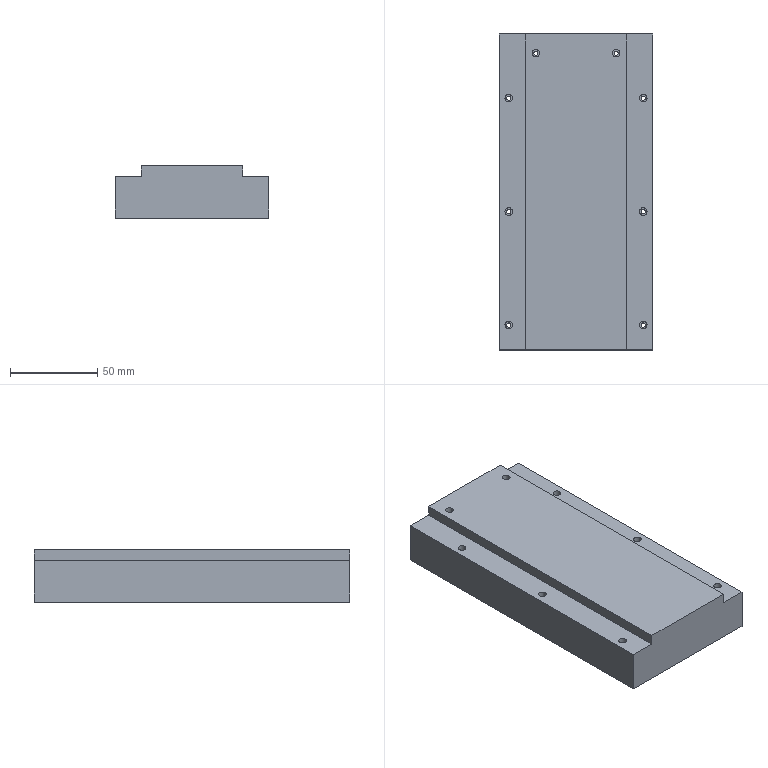NC program | NX | posted with a generic post | part box 88 x 181.05 x 30 mm
Lines 4247 to 5763 of 5763:
(PLANAR_MILL_3 , TOOL : D63_FACE_MILL)
N8480 T01 M6
N8482 G54
N8484 G17 G0 G90 X17.5 Y-153.525 S4500 M3
N8486 G43 Z20. H1
N8488 Z3.
N8490 G94 G1 Z0. F800.
N8492 Y-90.525
N8494 Y90.525
N8496 X-17.5
N8498 Y-90.525
N8500 Y-153.525
N8502 Z3.
N8504 G0 Z20.
N8506 M5
(PLANAR_MILL_4 , TOOL : D5-15-D6-50-3T-ROUGH)
N8508 T08 M6
N8510 G54
N8512 G17 G0 G90 X-25.04 Y69.397 S5000 M3
N8514 G43 Z20. H8
N8516 Z1.02
N8518 G94 G1 Z-0.98 F1500.
N8520 G3 X-27.04 Y71.397 R2.
N8522 G1 X-29.489
N8524 G3 X-30.889 Y69.997 R1.4
N8526 G1 Y67.548
N8528 G3 X-28.889 Y65.548 R2.
N8530 G1 Z1.02
N8532 G0 X-25.04 Y69.397 Z0.04
N8534 G1 Z-1.96
N8536 G3 X-27.04 Y71.397 R2.
N8538 G1 X-29.489
N8540 G3 X-30.889 Y69.997 R1.4
N8542 G1 Y67.548
N8544 G3 X-28.889 Y65.548 R2.
N8546 G1 Z0.04
N8548 G0 X-25.04 Y69.397 Z-0.94
N8550 G1 Z-2.94
N8552 G3 X-27.04 Y71.397 R2.
N8554 G1 X-29.489
N8556 G3 X-30.889 Y69.997 R1.4
N8558 G1 Y67.548
N8560 G3 X-28.889 Y65.548 R2.
N8562 G1 Z-0.94
N8564 G0 X-25.04 Y69.397 Z-1.92
N8566 G1 Z-3.92
N8568 G3 X-27.04 Y71.397 R2.
N8570 G1 X-29.489
N8572 G3 X-30.889 Y69.997 R1.4
N8574 G1 Y67.548
N8576 G3 X-28.889 Y65.548 R2.
N8578 G1 Z-1.92
N8580 G0 X-25.04 Y69.397 Z-2.9
N8582 G1 Z-4.9
N8584 G3 X-27.04 Y71.397 R2.
N8586 G1 X-29.489
N8588 G3 X-30.889 Y69.997 R1.4
N8590 G1 Y67.548
N8592 G3 X-28.889 Y65.548 R2.
N8594 G1 Z-2.9
N8596 G0 Z3.
N8598 Y28.051
N8600 Z1.02
N8602 G1 Z-0.98
N8604 G3 X-30.889 Y26.051 R2.
N8606 G1 Y23.602
N8608 G3 X-29.489 Y22.202 R1.4
N8610 G1 X-27.04
N8612 G3 X-25.04 Y24.202 R2.
N8614 G1 Z1.02
N8616 G0 X-28.889 Y28.051 Z0.04
N8618 G1 Z-1.96
N8620 G3 X-30.889 Y26.051 R2.
N8622 G1 Y23.602
N8624 G3 X-29.489 Y22.202 R1.4
N8626 G1 X-27.04
N8628 G3 X-25.04 Y24.202 R2.
N8630 G1 Z0.04
N8632 G0 X-28.889 Y28.051 Z-0.94
N8634 G1 Z-2.94
N8636 G3 X-30.889 Y26.051 R2.
N8638 G1 Y23.602
N8640 G3 X-29.489 Y22.202 R1.4
N8642 G1 X-27.04
N8644 G3 X-25.04 Y24.202 R2.
N8646 G1 Z-0.94
N8648 G0 X-28.889 Y28.051 Z-1.92
N8650 G1 Z-3.92
N8652 G3 X-30.889 Y26.051 R2.
N8654 G1 Y23.602
N8656 G3 X-29.489 Y22.202 R1.4
N8658 G1 X-27.04
N8660 G3 X-25.04 Y24.202 R2.
N8662 G1 Z-1.92
N8664 G0 X-28.889 Y28.051 Z-2.9
N8666 G1 Z-4.9
N8668 G3 X-30.889 Y26.051 R2.
N8670 G1 Y23.602
N8672 G3 X-29.489 Y22.202 R1.4
N8674 G1 X-27.04
N8676 G3 X-25.04 Y24.202 R2.
N8678 G1 Z-2.9
N8680 G0 Z3.
N8682 X24.773
N8684 Z1.02
N8686 G1 Z-0.98
N8688 G3 X26.773 Y22.202 R2.
N8690 G1 X29.222
N8692 G3 X30.622 Y23.602 R1.4
N8694 G1 Y26.051
N8696 G3 X28.622 Y28.051 R2.
N8698 G1 Z1.02
N8700 G0 X24.773 Y24.202 Z0.04
N8702 G1 Z-1.96
N8704 G3 X26.773 Y22.202 R2.
N8706 G1 X29.222
N8708 G3 X30.622 Y23.602 R1.4
N8710 G1 Y26.051
N8712 G3 X28.622 Y28.051 R2.
N8714 G1 Z0.04
N8716 G0 X24.773 Y24.202 Z-0.94
N8718 G1 Z-2.94
N8720 G3 X26.773 Y22.202 R2.
N8722 G1 X29.222
N8724 G3 X30.622 Y23.602 R1.4
N8726 G1 Y26.051
N8728 G3 X28.622 Y28.051 R2.
N8730 G1 Z-0.94
N8732 G0 X24.773 Y24.202 Z-1.92
N8734 G1 Z-3.92
N8736 G3 X26.773 Y22.202 R2.
N8738 G1 X29.222
N8740 G3 X30.622 Y23.602 R1.4
N8742 G1 Y26.051
N8744 G3 X28.622 Y28.051 R2.
N8746 G1 Z-1.92
N8748 G0 X24.773 Y24.202 Z-2.9
N8750 G1 Z-4.9
N8752 G3 X26.773 Y22.202 R2.
N8754 G1 X29.222
N8756 G3 X30.622 Y23.602 R1.4
N8758 G1 Y26.051
N8760 G3 X28.622 Y28.051 R2.
N8762 G1 Z-2.9
N8764 G0 Z3.
N8766 Y65.548
N8768 Z1.02
N8770 G1 Z-0.98
N8772 G3 X30.622 Y67.548 R2.
N8774 G1 Y69.997
N8776 G3 X29.222 Y71.397 R1.4
N8778 G1 X26.773
N8780 G3 X24.773 Y69.397 R2.
N8782 G1 Z1.02
N8784 G0 X28.622 Y65.548 Z0.04
N8786 G1 Z-1.96
N8788 G3 X30.622 Y67.548 R2.
N8790 G1 Y69.997
N8792 G3 X29.222 Y71.397 R1.4
N8794 G1 X26.773
N8796 G3 X24.773 Y69.397 R2.
N8798 G1 Z0.04
N8800 G0 X28.622 Y65.548 Z-0.94
N8802 G1 Z-2.94
N8804 G3 X30.622 Y67.548 R2.
N8806 G1 Y69.997
N8808 G3 X29.222 Y71.397 R1.4
N8810 G1 X26.773
N8812 G3 X24.773 Y69.397 R2.
N8814 G1 Z-0.94
N8816 G0 X28.622 Y65.548 Z-1.92
N8818 G1 Z-3.92
N8820 G3 X30.622 Y67.548 R2.
N8822 G1 Y69.997
N8824 G3 X29.222 Y71.397 R1.4
N8826 G1 X26.773
N8828 G3 X24.773 Y69.397 R2.
N8830 G1 Z-1.92
N8832 G0 X28.622 Y65.548 Z-2.9
N8834 G1 Z-4.9
N8836 G3 X30.622 Y67.548 R2.
N8838 G1 Y69.997
N8840 G3 X29.222 Y71.397 R1.4
N8842 G1 X26.773
N8844 G3 X24.773 Y69.397 R2.
N8846 G1 Z-2.9
N8848 G0 Z20.
(PLANAR_MILL_4_COPY , TOOL : D5-15-D6-50-3T-ROUGH)
N8850 X-13.196 Y12.175
N8852 Z1.5
N8854 G1 Z-0.5
N8856 G3 X-15.196 Y14.175 R2.
N8858 G1 X-18.072
N8860 G3 X-18.464 Y13.856 R0.4
N8862 G1 X-19.043 Y11.038
N8864 G3 X-17.487 Y8.676 R2.
N8866 G1 Z1.5
N8868 G0 Z20.
N8870 X17.487
N8872 Z1.5
N8874 G1 Z-0.5
N8876 G3 X19.043 Y11.038 R2.
N8878 G1 X18.464 Y13.856
N8880 G3 X18.072 Y14.175 R0.4
N8882 G1 X15.196
N8884 G3 X13.196 Y12.175 R2.
N8886 G1 Z1.5
N8888 G0 Z20.
N8890 X27.551 Y-68.925
N8892 Z1.5
N8894 G1 Z-0.5
N8896 G3 X29.551 Y-70.925 R2.
N8898 G1 X33.
N8900 G3 X33.4 Y-70.525 R0.4
N8902 G1 Y-67.076
N8904 G3 X31.4 Y-65.076 R2.
N8906 G1 Z1.5
N8908 G0 Z20.
N8910 X-31.4
N8912 Z1.5
N8914 G1 Z-0.5
N8916 G3 X-33.4 Y-67.076 R2.
N8918 G1 Y-70.525
N8920 G3 X-33. Y-70.925 R0.4
N8922 G1 X-29.551
N8924 G3 X-27.551 Y-68.925 R2.
N8926 G1 Z1.5
N8928 G0 Z20.
N8930 X-31.4 Y-65.076
N8932 Z1.
N8934 G1 Z-1.
N8936 G3 X-33.4 Y-67.076 R2.
N8938 G1 Y-70.525
N8940 G3 X-33. Y-70.925 R0.4
N8942 G1 X-29.551
N8944 G3 X-27.551 Y-68.925 R2.
N8946 G1 Z1.
N8948 G0 Z20.
N8950 X27.551
N8952 Z1.
N8954 G1 Z-1.
N8956 G3 X29.551 Y-70.925 R2.
N8958 G1 X33.
N8960 G3 X33.4 Y-70.525 R0.4
N8962 G1 Y-67.076
N8964 G3 X31.4 Y-65.076 R2.
N8966 G1 Z1.
N8968 G0 Z20.
N8970 X17.487 Y8.676
N8972 Z1.
N8974 G1 Z-1.
N8976 G3 X19.043 Y11.038 R2.
N8978 G1 X18.464 Y13.856
N8980 G3 X18.072 Y14.175 R0.4
N8982 G1 X15.196
N8984 G3 X13.196 Y12.175 R2.
N8986 G1 Z1.
N8988 G0 Z20.
N8990 X-13.196
N8992 Z1.
N8994 G1 Z-1.
N8996 G3 X-15.196 Y14.175 R2.
N8998 G1 X-18.072
N9000 G3 X-18.464 Y13.856 R0.4
N9002 G1 X-19.043 Y11.038
N9004 G3 X-17.487 Y8.676 R2.
N9006 G1 Z1.
N9008 G0 Z20.
N9010 X-13.196 Y12.175
N9012 Z0.5
N9014 G1 Z-1.5
N9016 G3 X-15.196 Y14.175 R2.
N9018 G1 X-18.072
N9020 G3 X-18.464 Y13.856 R0.4
N9022 G1 X-19.043 Y11.038
N9024 G3 X-17.487 Y8.676 R2.
N9026 G1 Z0.5
N9028 G0 Z20.
N9030 X17.487
N9032 Z0.5
N9034 G1 Z-1.5
N9036 G3 X19.043 Y11.038 R2.
N9038 G1 X18.464 Y13.856
N9040 G3 X18.072 Y14.175 R0.4
N9042 G1 X15.196
N9044 G3 X13.196 Y12.175 R2.
N9046 G1 Z0.5
N9048 G0 Z20.
N9050 X27.551 Y-68.925
N9052 Z0.5
N9054 G1 Z-1.5
N9056 G3 X29.551 Y-70.925 R2.
N9058 G1 X33.
N9060 G3 X33.4 Y-70.525 R0.4
N9062 G1 Y-67.076
N9064 G3 X31.4 Y-65.076 R2.
N9066 G1 Z0.5
N9068 G0 Z20.
N9070 X-31.4
N9072 Z0.5
N9074 G1 Z-1.5
N9076 G3 X-33.4 Y-67.076 R2.
N9078 G1 Y-70.525
N9080 G3 X-33. Y-70.925 R0.4
N9082 G1 X-29.551
N9084 G3 X-27.551 Y-68.925 R2.
N9086 G1 Z0.5
N9088 G0 Z20.
N9090 X-31.4 Y-65.076
N9092 Z0.4
N9094 G1 Z-1.6
N9096 G3 X-33.4 Y-67.076 R2.
N9098 G1 Y-70.525
N9100 G3 X-33. Y-70.925 R0.4
N9102 G1 X-29.551
N9104 G3 X-27.551 Y-68.925 R2.
N9106 G1 Z0.4
N9108 G0 Z20.
N9110 X27.551
N9112 Z0.4
N9114 G1 Z-1.6
N9116 G3 X29.551 Y-70.925 R2.
N9118 G1 X33.
N9120 G3 X33.4 Y-70.525 R0.4
N9122 G1 Y-67.076
N9124 G3 X31.4 Y-65.076 R2.
N9126 G1 Z0.4
N9128 G0 Z20.
N9130 X17.487 Y8.676
N9132 Z0.4
N9134 G1 Z-1.6
N9136 G3 X19.043 Y11.038 R2.
N9138 G1 X18.464 Y13.856
N9140 G3 X18.072 Y14.175 R0.4
N9142 G1 X15.196
N9144 G3 X13.196 Y12.175 R2.
N9146 G1 Z0.4
N9148 G0 Z20.
N9150 X-13.196
N9152 Z0.4
N9154 G1 Z-1.6
N9156 G3 X-15.196 Y14.175 R2.
N9158 G1 X-18.072
N9160 G3 X-18.464 Y13.856 R0.4
N9162 G1 X-19.043 Y11.038
N9164 G3 X-17.487 Y8.676 R2.
N9166 G1 Z0.4
N9168 G0 Z20.
(PLANAR_MILL_4_COPY_COPY , TOOL : D5-15-D6-50-3T-ROUGH)
N9170 X12.692 Y4.691
N9172 Z-0.696
N9174 G1 Z-2.696
N9176 G3 X14.248 Y7.053 R2.
N9178 G1 X13.668 Y9.871
N9180 G3 X13.277 Y10.19 R0.4
N9182 G1 X10.4
N9184 G3 X8.4 Y8.19 R2.
N9186 G1 Z-0.696
N9188 G0 X12.692 Y4.691 Z-1.691
N9190 G1 Z-3.691
N9192 G3 X14.248 Y7.053 R2.
N9194 G1 X13.668 Y9.871
N9196 G3 X13.277 Y10.19 R0.4
N9198 G1 X10.4
N9200 G3 X8.4 Y8.19 R2.
N9202 G1 Z-1.691
N9204 G0 X12.692 Y4.691 Z-2.687
N9206 G1 Z-4.687
N9208 G3 X14.248 Y7.053 R2.
N9210 G1 X13.668 Y9.871
N9212 G3 X13.277 Y10.19 R0.4
N9214 G1 X10.4
N9216 G3 X8.4 Y8.19 R2.
N9218 G1 Z-2.687
N9220 G0 X12.692 Y4.691 Z-3.683
N9222 G1 Z-5.683
N9224 G3 X14.248 Y7.053 R2.
N9226 G1 X13.668 Y9.871
N9228 G3 X13.277 Y10.19 R0.4
N9230 G1 X10.4
N9232 G3 X8.4 Y8.19 R2.
N9234 G1 Z-3.683
N9236 G0 X12.692 Y4.691 Z-4.678
N9238 G1 Z-6.678
N9240 G3 X14.248 Y7.053 R2.
N9242 G1 X13.668 Y9.871
N9244 G3 X13.277 Y10.19 R0.4
N9246 G1 X10.4
N9248 G3 X8.4 Y8.19 R2.
N9250 G1 Z-4.678
N9252 G0 X12.692 Y4.691 Z-5.674
N9254 G1 Z-7.674
N9256 G3 X14.248 Y7.053 R2.
N9258 G1 X13.668 Y9.871
N9260 G3 X13.277 Y10.19 R0.4
N9262 G1 X10.4
N9264 G3 X8.4 Y8.19 R2.
N9266 G1 Z-5.674
N9268 G0 X12.692 Y4.691 Z-6.67
N9270 G1 Z-8.67
N9272 G3 X14.248 Y7.053 R2.
N9274 G1 X13.668 Y9.871
N9276 G3 X13.277 Y10.19 R0.4
N9278 G1 X10.4
N9280 G3 X8.4 Y8.19 R2.
N9282 G1 Z-6.67
N9284 G0 X12.692 Y4.691 Z-7.665
N9286 G1 Z-9.665
N9288 G3 X14.248 Y7.053 R2.
N9290 G1 X13.668 Y9.871
N9292 G3 X13.277 Y10.19 R0.4
N9294 G1 X10.4
N9296 G3 X8.4 Y8.19 R2.
N9298 G1 Z-7.665
N9300 G0 X12.692 Y4.691 Z-8.661
N9302 G1 Z-10.661
N9304 G3 X14.248 Y7.053 R2.
N9306 G1 X13.668 Y9.871
N9308 G3 X13.277 Y10.19 R0.4
N9310 G1 X10.4
N9312 G3 X8.4 Y8.19 R2.
N9314 G1 Z-8.661
N9316 G0 X12.692 Y4.691 Z-9.657
N9318 G1 Z-11.657
N9320 G3 X14.248 Y7.053 R2.
N9322 G1 X13.668 Y9.871
N9324 G3 X13.277 Y10.19 R0.4
N9326 G1 X10.4
N9328 G3 X8.4 Y8.19 R2.
N9330 G1 Z-9.657
N9332 G0 X12.692 Y4.691 Z-10.652
N9334 G1 Z-12.652
N9336 G3 X14.248 Y7.053 R2.
N9338 G1 X13.668 Y9.871
N9340 G3 X13.277 Y10.19 R0.4
N9342 G1 X10.4
N9344 G3 X8.4 Y8.19 R2.
N9346 G1 Z-10.652
N9348 G0 X12.692 Y4.691 Z-11.648
N9350 G1 Z-13.648
N9352 G3 X14.248 Y7.053 R2.
N9354 G1 X13.668 Y9.871
N9356 G3 X13.277 Y10.19 R0.4
N9358 G1 X10.4
N9360 G3 X8.4 Y8.19 R2.
N9362 G1 Z-11.648
N9364 G0 X12.692 Y4.691 Z-12.643
N9366 G1 Z-14.643
N9368 G3 X14.248 Y7.053 R2.
N9370 G1 X13.668 Y9.871
N9372 G3 X13.277 Y10.19 R0.4
N9374 G1 X10.4
N9376 G3 X8.4 Y8.19 R2.
N9378 G1 Z-12.643
N9380 G0 X12.692 Y4.691 Z-13.639
N9382 G1 Z-15.639
N9384 G3 X14.248 Y7.053 R2.
N9386 G1 X13.668 Y9.871
N9388 G3 X13.277 Y10.19 R0.4
N9390 G1 X10.4
N9392 G3 X8.4 Y8.19 R2.
N9394 G1 Z-13.639
N9396 G0 X12.692 Y4.691 Z-14.635
N9398 G1 Z-16.635
N9400 G3 X14.248 Y7.053 R2.
N9402 G1 X13.668 Y9.871
N9404 G3 X13.277 Y10.19 R0.4
N9406 G1 X10.4
N9408 G3 X8.4 Y8.19 R2.
N9410 G1 Z-14.635
N9412 G0 X12.692 Y4.691 Z-15.63
N9414 G1 Z-17.63
N9416 G3 X14.248 Y7.053 R2.
N9418 G1 X13.668 Y9.871
N9420 G3 X13.277 Y10.19 R0.4
N9422 G1 X10.4
N9424 G3 X8.4 Y8.19 R2.
N9426 G1 Z-15.63
N9428 G0 X12.692 Y4.691 Z-16.626
N9430 G1 Z-18.626
N9432 G3 X14.248 Y7.053 R2.
N9434 G1 X13.668 Y9.871
N9436 G3 X13.277 Y10.19 R0.4
N9438 G1 X10.4
N9440 G3 X8.4 Y8.19 R2.
N9442 G1 Z-16.626
N9444 G0 X12.692 Y4.691 Z-17.622
N9446 G1 Z-19.622
N9448 G3 X14.248 Y7.053 R2.
N9450 G1 X13.668 Y9.871
N9452 G3 X13.277 Y10.19 R0.4
N9454 G1 X10.4
N9456 G3 X8.4 Y8.19 R2.
N9458 G1 Z-17.622
N9460 G0 X12.692 Y4.691 Z-18.617
N9462 G1 Z-20.617
N9464 G3 X14.248 Y7.053 R2.
N9466 G1 X13.668 Y9.871
N9468 G3 X13.277 Y10.19 R0.4
N9470 G1 X10.4
N9472 G3 X8.4 Y8.19 R2.
N9474 G1 Z-18.617
N9476 G0 X12.692 Y4.691 Z-19.613
N9478 G1 Z-21.613
N9480 G3 X14.248 Y7.053 R2.
N9482 G1 X13.668 Y9.871
N9484 G3 X13.277 Y10.19 R0.4
N9486 G1 X10.4
N9488 G3 X8.4 Y8.19 R2.
N9490 G1 Z-19.613
N9492 G0 X12.692 Y4.691 Z-20.609
N9494 G1 Z-22.609
N9496 G3 X14.248 Y7.053 R2.
N9498 G1 X13.668 Y9.871
N9500 G3 X13.277 Y10.19 R0.4
N9502 G1 X10.4
N9504 G3 X8.4 Y8.19 R2.
N9506 G1 Z-20.609
N9508 G0 X12.692 Y4.691 Z-21.604
N9510 G1 Z-23.604
N9512 G3 X14.248 Y7.053 R2.
N9514 G1 X13.668 Y9.871
N9516 G3 X13.277 Y10.19 R0.4
N9518 G1 X10.4
N9520 G3 X8.4 Y8.19 R2.
N9522 G1 Z-21.604
N9524 G0 X12.692 Y4.691 Z-22.6
N9526 G1 Z-24.6
N9528 G3 X14.248 Y7.053 R2.
N9530 G1 X13.668 Y9.871
N9532 G3 X13.277 Y10.19 R0.4
N9534 G1 X10.4
N9536 G3 X8.4 Y8.19 R2.
N9538 G1 Z-22.6
N9540 G0 Z1.3
N9542 X-8.4
N9544 Z-0.696
N9546 G1 Z-2.696
N9548 G3 X-10.4 Y10.19 R2.
N9550 G1 X-13.277
N9552 G3 X-13.668 Y9.871 R0.4
N9554 G1 X-14.248 Y7.053
N9556 G3 X-12.692 Y4.691 R2.
N9558 G1 Z-0.696
N9560 G0 X-8.4 Y8.19 Z-1.691
N9562 G1 Z-3.691
N9564 G3 X-10.4 Y10.19 R2.
N9566 G1 X-13.277
N9568 G3 X-13.668 Y9.871 R0.4
N9570 G1 X-14.248 Y7.053
N9572 G3 X-12.692 Y4.691 R2.
N9574 G1 Z-1.691
N9576 G0 X-8.4 Y8.19 Z-2.687
N9578 G1 Z-4.687
N9580 G3 X-10.4 Y10.19 R2.
N9582 G1 X-13.277
N9584 G3 X-13.668 Y9.871 R0.4
N9586 G1 X-14.248 Y7.053
N9588 G3 X-12.692 Y4.691 R2.
N9590 G1 Z-2.687
N9592 G0 X-8.4 Y8.19 Z-3.683
N9594 G1 Z-5.683
N9596 G3 X-10.4 Y10.19 R2.
N9598 G1 X-13.277
N9600 G3 X-13.668 Y9.871 R0.4
N9602 G1 X-14.248 Y7.053
N9604 G3 X-12.692 Y4.691 R2.
N9606 G1 Z-3.683
N9608 G0 X-8.4 Y8.19 Z-4.678
N9610 G1 Z-6.678
N9612 G3 X-10.4 Y10.19 R2.
N9614 G1 X-13.277
N9616 G3 X-13.668 Y9.871 R0.4
N9618 G1 X-14.248 Y7.053
N9620 G3 X-12.692 Y4.691 R2.
N9622 G1 Z-4.678
N9624 G0 X-8.4 Y8.19 Z-5.674
N9626 G1 Z-7.674
N9628 G3 X-10.4 Y10.19 R2.
N9630 G1 X-13.277
N9632 G3 X-13.668 Y9.871 R0.4
N9634 G1 X-14.248 Y7.053
N9636 G3 X-12.692 Y4.691 R2.
N9638 G1 Z-5.674
N9640 G0 X-8.4 Y8.19 Z-6.67
N9642 G1 Z-8.67
N9644 G3 X-10.4 Y10.19 R2.
N9646 G1 X-13.277
N9648 G3 X-13.668 Y9.871 R0.4
N9650 G1 X-14.248 Y7.053
N9652 G3 X-12.692 Y4.691 R2.
N9654 G1 Z-6.67
N9656 G0 X-8.4 Y8.19 Z-7.665
N9658 G1 Z-9.665
N9660 G3 X-10.4 Y10.19 R2.
N9662 G1 X-13.277
N9664 G3 X-13.668 Y9.871 R0.4
N9666 G1 X-14.248 Y7.053
N9668 G3 X-12.692 Y4.691 R2.
N9670 G1 Z-7.665
N9672 G0 X-8.4 Y8.19 Z-8.661
N9674 G1 Z-10.661
N9676 G3 X-10.4 Y10.19 R2.
N9678 G1 X-13.277
N9680 G3 X-13.668 Y9.871 R0.4
N9682 G1 X-14.248 Y7.053
N9684 G3 X-12.692 Y4.691 R2.
N9686 G1 Z-8.661
N9688 G0 X-8.4 Y8.19 Z-9.657
N9690 G1 Z-11.657
N9692 G3 X-10.4 Y10.19 R2.
N9694 G1 X-13.277
N9696 G3 X-13.668 Y9.871 R0.4
N9698 G1 X-14.248 Y7.053
N9700 G3 X-12.692 Y4.691 R2.
N9702 G1 Z-9.657
N9704 G0 X-8.4 Y8.19 Z-10.652
N9706 G1 Z-12.652
N9708 G3 X-10.4 Y10.19 R2.
N9710 G1 X-13.277
N9712 G3 X-13.668 Y9.871 R0.4
N9714 G1 X-14.248 Y7.053
N9716 G3 X-12.692 Y4.691 R2.
N9718 G1 Z-10.652
N9720 G0 X-8.4 Y8.19 Z-11.648
N9722 G1 Z-13.648
N9724 G3 X-10.4 Y10.19 R2.
N9726 G1 X-13.277
N9728 G3 X-13.668 Y9.871 R0.4
N9730 G1 X-14.248 Y7.053
N9732 G3 X-12.692 Y4.691 R2.
N9734 G1 Z-11.648
N9736 G0 X-8.4 Y8.19 Z-12.643
N9738 G1 Z-14.643
N9740 G3 X-10.4 Y10.19 R2.
N9742 G1 X-13.277
N9744 G3 X-13.668 Y9.871 R0.4
N9746 G1 X-14.248 Y7.053
N9748 G3 X-12.692 Y4.691 R2.
N9750 G1 Z-12.643
N9752 G0 X-8.4 Y8.19 Z-13.639
N9754 G1 Z-15.639
N9756 G3 X-10.4 Y10.19 R2.
N9758 G1 X-13.277
N9760 G3 X-13.668 Y9.871 R0.4
N9762 G1 X-14.248 Y7.053
N9764 G3 X-12.692 Y4.691 R2.
N9766 G1 Z-13.639
N9768 G0 X-8.4 Y8.19 Z-14.635
N9770 G1 Z-16.635
N9772 G3 X-10.4 Y10.19 R2.
N9774 G1 X-13.277
N9776 G3 X-13.668 Y9.871 R0.4
N9778 G1 X-14.248 Y7.053
N9780 G3 X-12.692 Y4.691 R2.
N9782 G1 Z-14.635
N9784 G0 X-8.4 Y8.19 Z-15.63
N9786 G1 Z-17.63
N9788 G3 X-10.4 Y10.19 R2.
N9790 G1 X-13.277
N9792 G3 X-13.668 Y9.871 R0.4
N9794 G1 X-14.248 Y7.053
N9796 G3 X-12.692 Y4.691 R2.
N9798 G1 Z-15.63
N9800 G0 X-8.4 Y8.19 Z-16.626
N9802 G1 Z-18.626
N9804 G3 X-10.4 Y10.19 R2.
N9806 G1 X-13.277
N9808 G3 X-13.668 Y9.871 R0.4
N9810 G1 X-14.248 Y7.053
N9812 G3 X-12.692 Y4.691 R2.
N9814 G1 Z-16.626
N9816 G0 X-8.4 Y8.19 Z-17.622
N9818 G1 Z-19.622
N9820 G3 X-10.4 Y10.19 R2.
N9822 G1 X-13.277
N9824 G3 X-13.668 Y9.871 R0.4
N9826 G1 X-14.248 Y7.053
N9828 G3 X-12.692 Y4.691 R2.
N9830 G1 Z-17.622
N9832 G0 X-8.4 Y8.19 Z-18.617
N9834 G1 Z-20.617
N9836 G3 X-10.4 Y10.19 R2.
N9838 G1 X-13.277
N9840 G3 X-13.668 Y9.871 R0.4
N9842 G1 X-14.248 Y7.053
N9844 G3 X-12.692 Y4.691 R2.
N9846 G1 Z-18.617
N9848 G0 X-8.4 Y8.19 Z-19.613
N9850 G1 Z-21.613
N9852 G3 X-10.4 Y10.19 R2.
N9854 G1 X-13.277
N9856 G3 X-13.668 Y9.871 R0.4
N9858 G1 X-14.248 Y7.053
N9860 G3 X-12.692 Y4.691 R2.
N9862 G1 Z-19.613
N9864 G0 X-8.4 Y8.19 Z-20.609
N9866 G1 Z-22.609
N9868 G3 X-10.4 Y10.19 R2.
N9870 G1 X-13.277
N9872 G3 X-13.668 Y9.871 R0.4
N9874 G1 X-14.248 Y7.053
N9876 G3 X-12.692 Y4.691 R2.
N9878 G1 Z-20.609
N9880 G0 X-8.4 Y8.19 Z-21.604
N9882 G1 Z-23.604
N9884 G3 X-10.4 Y10.19 R2.
N9886 G1 X-13.277
N9888 G3 X-13.668 Y9.871 R0.4
N9890 G1 X-14.248 Y7.053
N9892 G3 X-12.692 Y4.691 R2.
N9894 G1 Z-21.604
N9896 G0 X-8.4 Y8.19 Z-22.6
N9898 G1 Z-24.6
N9900 G3 X-10.4 Y10.19 R2.
N9902 G1 X-13.277
N9904 G3 X-13.668 Y9.871 R0.4
N9906 G1 X-14.248 Y7.053
N9908 G3 X-12.692 Y4.691 R2.
N9910 G1 Z-22.6
N9912 G0 Z1.3
N9914 X-26.166 Y-60.822
N9916 Z-0.696
N9918 G1 Z-2.696
N9920 G3 X-28.528 Y-62.378 R2.
N9922 G1 X-29.364 Y-66.444
N9924 G3 X-28.972 Y-66.925 R0.4
N9926 G1 X-24.82
N9928 G3 X-22.82 Y-64.925 R2.
N9930 G1 Z-0.696
N9932 G0 X-26.166 Y-60.822 Z-1.691
N9934 G1 Z-3.691
N9936 G3 X-28.528 Y-62.378 R2.
N9938 G1 X-29.364 Y-66.444
N9940 G3 X-28.972 Y-66.925 R0.4
N9942 G1 X-24.82
N9944 G3 X-22.82 Y-64.925 R2.
N9946 G1 Z-1.691
N9948 G0 X-26.166 Y-60.822 Z-2.687
N9950 G1 Z-4.687
N9952 G3 X-28.528 Y-62.378 R2.
N9954 G1 X-29.364 Y-66.444
N9956 G3 X-28.972 Y-66.925 R0.4
N9958 G1 X-24.82
N9960 G3 X-22.82 Y-64.925 R2.
N9962 G1 Z-2.687
N9964 G0 X-26.166 Y-60.822 Z-3.683
N9966 G1 Z-5.683
N9968 G3 X-28.528 Y-62.378 R2.
N9970 G1 X-29.364 Y-66.444
N9972 G3 X-28.972 Y-66.925 R0.4
N9974 G1 X-24.82
N9976 G3 X-22.82 Y-64.925 R2.
N9978 G1 Z-3.683
N9980 G0 X-26.166 Y-60.822 Z-4.678
N9982 G1 Z-6.678
N9984 G3 X-28.528 Y-62.378 R2.
N9986 G1 X-29.364 Y-66.444
N9988 G3 X-28.972 Y-66.925 R0.4
N9990 G1 X-24.82
N9992 G3 X-22.82 Y-64.925 R2.
N9994 G1 Z-4.678
N9996 G0 X-26.166 Y-60.822 Z-5.674
N9998 G1 Z-7.674
N10000 G3 X-28.528 Y-62.378 R2.
N10002 G1 X-29.364 Y-66.444
N10004 G3 X-28.972 Y-66.925 R0.4
N10006 G1 X-24.82
N10008 G3 X-22.82 Y-64.925 R2.
N10010 G1 Z-5.674
N10012 G0 X-26.166 Y-60.822 Z-6.67
N10014 G1 Z-8.67
N10016 G3 X-28.528 Y-62.378 R2.
N10018 G1 X-29.364 Y-66.444
N10020 G3 X-28.972 Y-66.925 R0.4
N10022 G1 X-24.82
N10024 G3 X-22.82 Y-64.925 R2.
N10026 G1 Z-6.67
N10028 G0 X-26.166 Y-60.822 Z-7.665
N10030 G1 Z-9.665
N10032 G3 X-28.528 Y-62.378 R2.
N10034 G1 X-29.364 Y-66.444
N10036 G3 X-28.972 Y-66.925 R0.4
N10038 G1 X-24.82
N10040 G3 X-22.82 Y-64.925 R2.
N10042 G1 Z-7.665
N10044 G0 X-26.166 Y-60.822 Z-8.661
N10046 G1 Z-10.661
N10048 G3 X-28.528 Y-62.378 R2.
N10050 G1 X-29.364 Y-66.444
N10052 G3 X-28.972 Y-66.925 R0.4
N10054 G1 X-24.82
N10056 G3 X-22.82 Y-64.925 R2.
N10058 G1 Z-8.661
N10060 G0 X-26.166 Y-60.822 Z-9.657
N10062 G1 Z-11.657
N10064 G3 X-28.528 Y-62.378 R2.
N10066 G1 X-29.364 Y-66.444
N10068 G3 X-28.972 Y-66.925 R0.4
N10070 G1 X-24.82
N10072 G3 X-22.82 Y-64.925 R2.
N10074 G1 Z-9.657
N10076 G0 X-26.166 Y-60.822 Z-10.652
N10078 G1 Z-12.652
N10080 G3 X-28.528 Y-62.378 R2.
N10082 G1 X-29.364 Y-66.444
N10084 G3 X-28.972 Y-66.925 R0.4
N10086 G1 X-24.82
N10088 G3 X-22.82 Y-64.925 R2.
N10090 G1 Z-10.652
N10092 G0 X-26.166 Y-60.822 Z-11.648
N10094 G1 Z-13.648
N10096 G3 X-28.528 Y-62.378 R2.
N10098 G1 X-29.364 Y-66.444
N10100 G3 X-28.972 Y-66.925 R0.4
N10102 G1 X-24.82
N10104 G3 X-22.82 Y-64.925 R2.
N10106 G1 Z-11.648
N10108 G0 X-26.166 Y-60.822 Z-12.643
N10110 G1 Z-14.643
N10112 G3 X-28.528 Y-62.378 R2.
N10114 G1 X-29.364 Y-66.444
N10116 G3 X-28.972 Y-66.925 R0.4
N10118 G1 X-24.82
N10120 G3 X-22.82 Y-64.925 R2.
N10122 G1 Z-12.643
N10124 G0 X-26.166 Y-60.822 Z-13.639
N10126 G1 Z-15.639
N10128 G3 X-28.528 Y-62.378 R2.
N10130 G1 X-29.364 Y-66.444
N10132 G3 X-28.972 Y-66.925 R0.4
N10134 G1 X-24.82
N10136 G3 X-22.82 Y-64.925 R2.
N10138 G1 Z-13.639
N10140 G0 X-26.166 Y-60.822 Z-14.635
N10142 G1 Z-16.635
N10144 G3 X-28.528 Y-62.378 R2.
N10146 G1 X-29.364 Y-66.444
N10148 G3 X-28.972 Y-66.925 R0.4
N10150 G1 X-24.82
N10152 G3 X-22.82 Y-64.925 R2.
N10154 G1 Z-14.635
N10156 G0 X-26.166 Y-60.822 Z-15.63
N10158 G1 Z-17.63
N10160 G3 X-28.528 Y-62.378 R2.
N10162 G1 X-29.364 Y-66.444
N10164 G3 X-28.972 Y-66.925 R0.4
N10166 G1 X-24.82
N10168 G3 X-22.82 Y-64.925 R2.
N10170 G1 Z-15.63
N10172 G0 X-26.166 Y-60.822 Z-16.626
N10174 G1 Z-18.626
N10176 G3 X-28.528 Y-62.378 R2.
N10178 G1 X-29.364 Y-66.444
N10180 G3 X-28.972 Y-66.925 R0.4
N10182 G1 X-24.82
N10184 G3 X-22.82 Y-64.925 R2.
N10186 G1 Z-16.626
N10188 G0 X-26.166 Y-60.822 Z-17.622
N10190 G1 Z-19.622
N10192 G3 X-28.528 Y-62.378 R2.
N10194 G1 X-29.364 Y-66.444
N10196 G3 X-28.972 Y-66.925 R0.4
N10198 G1 X-24.82
N10200 G3 X-22.82 Y-64.925 R2.
N10202 G1 Z-17.622
N10204 G0 X-26.166 Y-60.822 Z-18.617
N10206 G1 Z-20.617
N10208 G3 X-28.528 Y-62.378 R2.
N10210 G1 X-29.364 Y-66.444
N10212 G3 X-28.972 Y-66.925 R0.4
N10214 G1 X-24.82
N10216 G3 X-22.82 Y-64.925 R2.
N10218 G1 Z-18.617
N10220 G0 X-26.166 Y-60.822 Z-19.613
N10222 G1 Z-21.613
N10224 G3 X-28.528 Y-62.378 R2.
N10226 G1 X-29.364 Y-66.444
N10228 G3 X-28.972 Y-66.925 R0.4
N10230 G1 X-24.82
N10232 G3 X-22.82 Y-64.925 R2.
N10234 G1 Z-19.613
N10236 G0 X-26.166 Y-60.822 Z-20.609
N10238 G1 Z-22.609
N10240 G3 X-28.528 Y-62.378 R2.
N10242 G1 X-29.364 Y-66.444
N10244 G3 X-28.972 Y-66.925 R0.4
N10246 G1 X-24.82
N10248 G3 X-22.82 Y-64.925 R2.
N10250 G1 Z-20.609
N10252 G0 X-26.166 Y-60.822 Z-21.604
N10254 G1 Z-23.604
N10256 G3 X-28.528 Y-62.378 R2.
N10258 G1 X-29.364 Y-66.444
N10260 G3 X-28.972 Y-66.925 R0.4
N10262 G1 X-24.82
N10264 G3 X-22.82 Y-64.925 R2.
N10266 G1 Z-21.604
N10268 G0 X-26.166 Y-60.822 Z-22.6
N10270 G1 Z-24.6
N10272 G3 X-28.528 Y-62.378 R2.
N10274 G1 X-29.364 Y-66.444
N10276 G3 X-28.972 Y-66.925 R0.4
N10278 G1 X-24.82
N10280 G3 X-22.82 Y-64.925 R2.
N10282 G1 Z-22.6
N10284 G0 Z1.3
N10286 X22.82
N10288 Z-0.696
N10290 G1 Z-2.696
N10292 G3 X24.82 Y-66.925 R2.
N10294 G1 X28.972
N10296 G3 X29.364 Y-66.444 R0.4
N10298 G1 X28.528 Y-62.378
N10300 G3 X26.166 Y-60.822 R2.
N10302 G1 Z-0.696
N10304 G0 X22.82 Y-64.925 Z-1.691
N10306 G1 Z-3.691
N10308 G3 X24.82 Y-66.925 R2.
N10310 G1 X28.972
N10312 G3 X29.364 Y-66.444 R0.4
N10314 G1 X28.528 Y-62.378
N10316 G3 X26.166 Y-60.822 R2.
N10318 G1 Z-1.691
N10320 G0 X22.82 Y-64.925 Z-2.687
N10322 G1 Z-4.687
N10324 G3 X24.82 Y-66.925 R2.
N10326 G1 X28.972
N10328 G3 X29.364 Y-66.444 R0.4
N10330 G1 X28.528 Y-62.378
N10332 G3 X26.166 Y-60.822 R2.
N10334 G1 Z-2.687
N10336 G0 X22.82 Y-64.925 Z-3.683
N10338 G1 Z-5.683
N10340 G3 X24.82 Y-66.925 R2.
N10342 G1 X28.972
N10344 G3 X29.364 Y-66.444 R0.4
N10346 G1 X28.528 Y-62.378
N10348 G3 X26.166 Y-60.822 R2.
N10350 G1 Z-3.683
N10352 G0 X22.82 Y-64.925 Z-4.678
N10354 G1 Z-6.678
N10356 G3 X24.82 Y-66.925 R2.
N10358 G1 X28.972
N10360 G3 X29.364 Y-66.444 R0.4
N10362 G1 X28.528 Y-62.378
N10364 G3 X26.166 Y-60.822 R2.
N10366 G1 Z-4.678
N10368 G0 X22.82 Y-64.925 Z-5.674
N10370 G1 Z-7.674
N10372 G3 X24.82 Y-66.925 R2.
N10374 G1 X28.972
N10376 G3 X29.364 Y-66.444 R0.4
N10378 G1 X28.528 Y-62.378
N10380 G3 X26.166 Y-60.822 R2.
N10382 G1 Z-5.674
N10384 G0 X22.82 Y-64.925 Z-6.67
N10386 G1 Z-8.67
N10388 G3 X24.82 Y-66.925 R2.
N10390 G1 X28.972
N10392 G3 X29.364 Y-66.444 R0.4
N10394 G1 X28.528 Y-62.378
N10396 G3 X26.166 Y-60.822 R2.
N10398 G1 Z-6.67
N10400 G0 X22.82 Y-64.925 Z-7.665
N10402 G1 Z-9.665
N10404 G3 X24.82 Y-66.925 R2.
N10406 G1 X28.972
N10408 G3 X29.364 Y-66.444 R0.4
N10410 G1 X28.528 Y-62.378
N10412 G3 X26.166 Y-60.822 R2.
N10414 G1 Z-7.665
N10416 G0 X22.82 Y-64.925 Z-8.661
N10418 G1 Z-10.661
N10420 G3 X24.82 Y-66.925 R2.
N10422 G1 X28.972
N10424 G3 X29.364 Y-66.444 R0.4
N10426 G1 X28.528 Y-62.378
N10428 G3 X26.166 Y-60.822 R2.
N10430 G1 Z-8.661
N10432 G0 X22.82 Y-64.925 Z-9.657
N10434 G1 Z-11.657
N10436 G3 X24.82 Y-66.925 R2.
N10438 G1 X28.972
N10440 G3 X29.364 Y-66.444 R0.4
N10442 G1 X28.528 Y-62.378
N10444 G3 X26.166 Y-60.822 R2.
N10446 G1 Z-9.657
N10448 G0 X22.82 Y-64.925 Z-10.652
N10450 G1 Z-12.652
N10452 G3 X24.82 Y-66.925 R2.
N10454 G1 X28.972
N10456 G3 X29.364 Y-66.444 R0.4
N10458 G1 X28.528 Y-62.378
N10460 G3 X26.166 Y-60.822 R2.
N10462 G1 Z-10.652
N10464 G0 X22.82 Y-64.925 Z-11.648
N10466 G1 Z-13.648
N10468 G3 X24.82 Y-66.925 R2.
N10470 G1 X28.972
N10472 G3 X29.364 Y-66.444 R0.4
N10474 G1 X28.528 Y-62.378
N10476 G3 X26.166 Y-60.822 R2.
N10478 G1 Z-11.648
N10480 G0 X22.82 Y-64.925 Z-12.643
N10482 G1 Z-14.643
N10484 G3 X24.82 Y-66.925 R2.
N10486 G1 X28.972
N10488 G3 X29.364 Y-66.444 R0.4
N10490 G1 X28.528 Y-62.378
N10492 G3 X26.166 Y-60.822 R2.
N10494 G1 Z-12.643
N10496 G0 X22.82 Y-64.925 Z-13.639
N10498 G1 Z-15.639
N10500 G3 X24.82 Y-66.925 R2.
N10502 G1 X28.972
N10504 G3 X29.364 Y-66.444 R0.4
N10506 G1 X28.528 Y-62.378
N10508 G3 X26.166 Y-60.822 R2.
N10510 G1 Z-13.639
N10512 G0 X22.82 Y-64.925 Z-14.635
N10514 G1 Z-16.635
N10516 G3 X24.82 Y-66.925 R2.
N10518 G1 X28.972
N10520 G3 X29.364 Y-66.444 R0.4
N10522 G1 X28.528 Y-62.378
N10524 G3 X26.166 Y-60.822 R2.
N10526 G1 Z-14.635
N10528 G0 X22.82 Y-64.925 Z-15.63
N10530 G1 Z-17.63
N10532 G3 X24.82 Y-66.925 R2.
N10534 G1 X28.972
N10536 G3 X29.364 Y-66.444 R0.4
N10538 G1 X28.528 Y-62.378
N10540 G3 X26.166 Y-60.822 R2.
N10542 G1 Z-15.63
N10544 G0 X22.82 Y-64.925 Z-16.626
N10546 G1 Z-18.626
N10548 G3 X24.82 Y-66.925 R2.
N10550 G1 X28.972
N10552 G3 X29.364 Y-66.444 R0.4
N10554 G1 X28.528 Y-62.378
N10556 G3 X26.166 Y-60.822 R2.
N10558 G1 Z-16.626
N10560 G0 X22.82 Y-64.925 Z-17.622
N10562 G1 Z-19.622
N10564 G3 X24.82 Y-66.925 R2.
N10566 G1 X28.972
N10568 G3 X29.364 Y-66.444 R0.4
N10570 G1 X28.528 Y-62.378
N10572 G3 X26.166 Y-60.822 R2.
N10574 G1 Z-17.622
N10576 G0 X22.82 Y-64.925 Z-18.617
N10578 G1 Z-20.617
N10580 G3 X24.82 Y-66.925 R2.
N10582 G1 X28.972
N10584 G3 X29.364 Y-66.444 R0.4
N10586 G1 X28.528 Y-62.378
N10588 G3 X26.166 Y-60.822 R2.
N10590 G1 Z-18.617
N10592 G0 X22.82 Y-64.925 Z-19.613
N10594 G1 Z-21.613
N10596 G3 X24.82 Y-66.925 R2.
N10598 G1 X28.972
N10600 G3 X29.364 Y-66.444 R0.4
N10602 G1 X28.528 Y-62.378
N10604 G3 X26.166 Y-60.822 R2.
N10606 G1 Z-19.613
N10608 G0 X22.82 Y-64.925 Z-20.609
N10610 G1 Z-22.609
N10612 G3 X24.82 Y-66.925 R2.
N10614 G1 X28.972
N10616 G3 X29.364 Y-66.444 R0.4
N10618 G1 X28.528 Y-62.378
N10620 G3 X26.166 Y-60.822 R2.
N10622 G1 Z-20.609
N10624 G0 X22.82 Y-64.925 Z-21.604
N10626 G1 Z-23.604
N10628 G3 X24.82 Y-66.925 R2.
N10630 G1 X28.972
N10632 G3 X29.364 Y-66.444 R0.4
N10634 G1 X28.528 Y-62.378
N10636 G3 X26.166 Y-60.822 R2.
N10638 G1 Z-21.604
N10640 G0 X22.82 Y-64.925 Z-22.6
N10642 G1 Z-24.6
N10644 G3 X24.82 Y-66.925 R2.
N10646 G1 X28.972
N10648 G3 X29.364 Y-66.444 R0.4
N10650 G1 X28.528 Y-62.378
N10652 G3 X26.166 Y-60.822 R2.
N10654 G1 Z-22.6
N10656 G0 Z20.
(PLANAR_MILL_6_COPY_1_COPY , TOOL : D5-15-D6-50-3T-ROUGH)
N10658 X-22.215 Y-26.723 S5500
N10660 Z0.4
N10662 G1 Z-1.6 F1000.
N10664 G3 X-24.577 Y-28.279 R2.
N10666 G1 X-30.9 Y-59.021
N10668 Y-68.425
N10670 X30.9
N10672 Y-59.021
N10674 X16.36 Y11.675
N10676 X-16.36
N10678 X-24.577 Y-28.279
N10680 G3 X-23.021 Y-30.641 R2.
N10682 G1 X-24.664 Y-26.219
N10684 G3 X-27.026 Y-27.775 R2.
N10686 G1 X-33.392 Y-58.727
N10688 X-33.4 Y-58.808
N10690 Y-70.525
N10692 G3 X-33. Y-70.925 R0.4
N10694 G1 X33.
N10696 G3 X33.4 Y-70.525 R0.4
N10698 G1 Y-58.808
N10700 X33.392 Y-58.727
N10702 X18.464 Y13.856
N10704 G3 X18.072 Y14.175 R0.4
N10706 G1 X-18.072
N10708 G3 X-18.464 Y13.856 R0.4
N10710 G1 X-27.026 Y-27.775
N10712 G3 X-25.47 Y-30.137 R2.
N10714 G1 Z0.4
N10716 G0 Z20.
N10718 M5
(PLANAR_MILL_8 , TOOL : D6-18-D6-50-3T-FINISH)
N10720 T09 M6
N10722 G54
N10724 G17 G0 G90 X-47.5 Y-91.525 S4500 M3
N10726 G43 Z20. H9
N10728 Z-3.
N10730 G94 G1 Z-5. F700.
N10732 G3 X-45.5 Y-89.525 R2.
N10734 G1 Y86.525
N10736 G2 X-39.5 Y92.525 R6.
N10738 G1 X39.5
N10740 G2 X45.5 Y86.525 R6.
N10742 G1 Y-89.525
N10744 G2 X42.5 Y-92.525 R3.
N10746 G1 X-42.5
N10748 G2 X-45.5 Y-89.525 R3.
N10750 G3 X-47.5 Y-87.525 R2.
N10752 G1 Z-3.
N10754 G0 Z20.
(PLANAR_MILL_5 , TOOL : D6-18-D6-50-3T-FINISH)
N10756 X-14. Y46.799
N10758 Z-2.
N10760 G1 Z-5.
N10762 X-20.
N10764 Y24.977
N10766 G3 X-19.124 Y22.84 R3.045
N10768 X-18.921 Y22.652 R2.982
N10770 G1 X-29.489
N10772 G2 X-30.439 Y23.602 R0.95
N10774 G1 Y69.997
N10776 G2 X-29.489 Y70.947 R0.95
N10778 G1 X-19.551
N10780 G3 X-20. Y69.356 R3.045
N10782 G1 Y46.799
N10784 X-23.6
N10786 Y26.252
N10788 X-26.839
N10790 Y67.347
N10792 X-23.6
N10794 Y46.799
N10796 X-14.
N10798 Z-2.
N10800 G0 Z20.
N10802 X14.
N10804 Z-2.
N10806 G1 Z-5.
N10808 X20.
N10810 Y69.356
N10812 G3 X19.551 Y70.947 R3.045
N10814 G1 X29.222
N10816 G2 X30.172 Y69.997 R0.95
N10818 G1 Y23.602
N10820 G2 X29.222 Y22.652 R0.95
N10822 G1 X18.921
N10824 G3 X19.124 Y22.84 R2.982
N10826 X20. Y24.977 R3.045
N10828 G1 Y46.799
N10830 X23.6
N10832 Y67.347
N10834 X26.572
N10836 Y26.252
N10838 X23.6
N10840 Y46.799
N10842 X14.
N10844 Z-2.
N10846 G0 Z20.
(PLANAR_MILL_5_COPY , TOOL : D6-18-D6-50-3T-FINISH)
N10848 X-27.489 Y68.997
N10850 Z-3.
N10852 G1 Z-5.
N10854 G3 X-29.489 Y70.997 R2.
N10856 X-30.489 Y69.997 R1.
N10858 G1 Y23.602
N10860 G3 X-29.489 Y22.602 R1.
N10862 G1 X29.222
N10864 G3 X30.222 Y23.602 R1.
N10866 G1 Y69.997
N10868 G3 X29.222 Y70.997 R1.
N10870 G1 X-29.489
N10872 G3 X-30.489 Y69.997 R1.
N10874 G1 X-27.489 Y68.997
N10876 G3 X-29.489 Y70.997 R2.
N10878 X-30.489 Y69.997 R1.
N10880 G1 Y23.602
N10882 G3 X-29.489 Y22.602 R1.
N10884 G1 X29.222
N10886 G3 X30.222 Y23.602 R1.
N10888 G1 Y69.997
N10890 G3 X29.222 Y70.997 R1.
N10892 G1 X-29.489
N10894 G3 X-30.489 Y69.997 R1.
N10896 G1 X-28.489 Y68.997
N10898 Z-3.
N10900 G0 Z20.
(PLANAR_MILL_6 , TOOL : D6-18-D6-50-3T-FINISH)
N10902 X-20.636 Y-26.74
N10904 Z0.3
N10906 G1 Z-1.7
N10908 G3 X-22.998 Y-28.296 R2.
N10910 G1 X-29.35 Y-59.179
N10912 Y-66.875
N10914 X29.35
N10916 Y-59.179
N10918 X15.096 Y10.125
N10920 X-15.096
N10922 X-22.998 Y-28.296
N10924 G3 X-21.442 Y-30.658 R2.
N10926 G1 X-24.163 Y-26.015
N10928 G3 X-26.525 Y-27.571 R2.
N10930 G1 X-32.95 Y-58.813
N10932 Y-70.475
N10934 X32.95
N10936 Y-58.813
N10938 X18.031 Y13.725
N10940 X-18.031
N10942 X-26.525 Y-27.571
N10944 G3 X-24.968 Y-29.933 R2.
N10946 G1 Z0.3
N10948 G0 Z20.
(PLANAR_MILL_6_COPY_1 , TOOL : D6-18-D6-50-3T-FINISH)
N10950 X-24.354 Y-26.699
N10952 Z0.3
N10954 G1 Z-1.7
N10956 G3 X-26.716 Y-28.255 R2.
N10958 G1 X-33. Y-58.808
N10960 Y-70.525
N10962 X33.
N10964 Y-58.808
N10966 X18.072 Y13.775
N10968 X-18.072
N10970 X-26.716 Y-28.255
N10972 G3 X-25.16 Y-30.617 R2.
N10974 G1 Z0.3
N10976 G0 Z20.
(PLANAR_MILL_6_COPY , TOOL : D6-18-D6-50-3T-FINISH)
N10978 X-43.75 Y-94.525
N10980 Z1.
N10982 G1 Z-1.
N10984 Y-89.525
N10986 Y78.225
N10988 G2 X-36.75 Y85.225 R7.
N10990 G1 X36.75
N10992 G2 X43.75 Y78.225 R7.
N10994 G1 Y-89.525
N10996 Y-94.525
N10998 Z1.
N11000 G0 Z20.
(PLANAR_MILL_6_COPY_COPY , TOOL : D6-18-D6-50-3T-FINISH)
N11002 X44.5 Y87.525
N11004 Z1.
N11006 G1 Z-1.
N11008 X39.5
N11010 X-39.5
N11012 X-44.5
N11014 Z1.
N11016 G0 Z20.
N11018 M5
(PLANAR_MILL_7_COPY , TOOL : D6-18-D6-50-3T-ROUGH)
N11020 T12 M6
N11022 G54
N11024 G17 G0 G90 X-11.277 Y7.79 S4500 M3
N11026 G43 Z20. H12
N11028 Z-22.7
N11030 G94 G1 Z-24.7 F700.
N11032 G3 X-13.277 Y9.79 R2.
N11034 G1 X-28.972 Y-66.525
N11036 X28.972
N11038 X13.277 Y9.79
N11040 X-13.277
N11042 G3 X-11.72 Y7.428 R2.
N11044 G1 X-11.277 Y7.79
N11046 G3 X-13.277 Y9.79 R2.
N11048 G1 X-28.972 Y-66.525
N11050 X28.972
N11052 X13.277 Y9.79
N11054 X-13.277
N11056 G3 X-11.72 Y7.428 R2.
N11058 G1 X-11.277 Y7.79
N11060 G3 X-13.277 Y9.79 R2.
N11062 G1 X-28.972 Y-66.525
N11064 X28.972
N11066 X13.277 Y9.79
N11068 X-13.277
N11070 G3 X-11.72 Y7.428 R2.
N11072 G1 Z-22.7
N11074 G0 Z20.
N11076 M5
(DRILLING_2 , TOOL : CHAMFER_D6-90DEG)
N11078 T04 M6
N11080 G54
N11082 G17 G0 G90 X32.252 Y-54.525 S3000 M3
N11084 G43 Z20. H4
N11086 G94 G81 G99 Z-2.7 F250. R1.3
N11088 X25.054 Y-19.525
N11090 X18.884 Y10.475
N11092 X-18.884
N11094 X-25.054 Y-19.525
N11096 X-32.252 Y-54.525
N11098 G80
N11100 G0 X-32.252 Y-54.525 Z20.
(DRILLING_3 , TOOL : CHAMFER_D6-90DEG)
N11102 X-38.5 Y-76.225
N11104 G81 Z-1.2 F250. R3.
N11106 Y-11.225
N11108 Y53.775
N11110 X-23. Y79.525
N11112 X23.
N11114 X38.5 Y53.775
N11116 Y-11.225
N11118 Y-76.225
N11120 G80
N11122 G0 X38.5 Y-76.225 Z20.
(PLANAR_CHAMFER_MILL , TOOL : CHAMFER_D6-90DEG)
N11124 X-41.755 Y-90.164 S4500
N11126 Z2.2
N11128 G1 Z-0.8 F1000.
N11130 G41 X-41.58 Y-89.696 D4
N11132 X-41.528 Y-89.617
N11134 X-41.55 Y-89.525
N11136 Y78.225
N11138 G2 X-36.75 Y83.025 R4.8
N11140 G1 X36.75
N11142 G2 X41.55 Y78.225 R4.8
N11144 G1 Y-89.525
N11146 X41.528 Y-89.617
N11148 X41.58 Y-89.696
N11150 G40
N11152 X41.755 Y-90.164
N11154 Z2.2
N11156 G0 Z20.
(PLANAR_CHAMFER_MILL_4 , TOOL : CHAMFER_D6-90DEG)
N11158 X-44.705
N11160 Z0.
N11162 G1 Z-3.
N11164 G41 X-44.53 Y-89.696
N11166 X-44.478 Y-89.617
N11168 X-44.5 Y-89.525
N11170 Y86.525
N11172 G2 X-39.5 Y91.525 R5.
N11174 G1 X39.5
N11176 G2 X44.5 Y86.525 R5.
N11178 G1 Y-89.525
N11180 X44.478 Y-89.617
N11182 X44.53 Y-89.696
N11184 G40
N11186 X44.705 Y-90.164
N11188 Z0.
N11190 G0 Z20.
(PLANAR_CHAMFER_MILL_1 , TOOL : CHAMFER_D6-90DEG)
N11192 X-28.287 Y-27.476
N11194 Z1.5
N11196 G1 Z-1.5
N11198 G41 X-28.552 Y-27.9
N11200 X-28.619 Y-27.967
N11202 X-28.616 Y-28.061
N11204 X-34.861 Y-58.425
N11206 G3 X-34.9 Y-58.808 R1.9
N11208 G1 Y-70.525
N11210 G3 X-33. Y-72.425 R1.9
N11212 G1 X33.
N11214 G3 X34.9 Y-70.525 R1.9
N11216 G1 Y-58.808
N11218 G3 X34.861 Y-58.425 R1.9
N11220 G1 X19.933 Y14.158
N11222 G3 X18.072 Y15.675 R1.9
N11224 G1 X-18.072
N11226 G3 X-19.933 Y14.158 R1.9
N11228 G1 X-28.616 Y-28.061
N11230 X-28.656 Y-28.146
N11232 X-28.621 Y-28.234
N11234 G40
N11236 X-28.544 Y-28.728
N11238 Z1.5
N11240 G0 Z20.
(PLANAR_CHAMFER_MILL_3 , TOOL : CHAMFER_D6-90DEG)
N11242 X-22.795 Y-27.578
N11244 Z0.3
N11246 G1 Z-2.7
N11248 G41 X-23.06 Y-28.002
N11250 X-23.127 Y-28.069
N11252 X-23.124 Y-28.163
N11254 X-30.931 Y-66.122
N11256 G3 X-28.972 Y-68.525 R2.
N11258 G1 X28.972
N11260 G3 X30.931 Y-66.122 R2.
N11262 G1 X15.236 Y10.193
N11264 G3 X13.277 Y11.79 R2.
N11266 G1 X-13.277
N11268 G3 X-15.236 Y10.193 R2.
N11270 G1 X-23.124 Y-28.163
N11272 X-23.164 Y-28.249
N11274 X-23.129 Y-28.336
N11276 G40
N11278 X-23.052 Y-28.83
N11280 Z0.3
N11282 G0 Z20.
(PLANAR_CHAMFER_MILL_2 , TOOL : CHAMFER_D6-90DEG)
N11284 X-0.772 Y20.807
N11286 Z2.
N11288 G1 Z-1.
N11290 G41 X-0.304 Y20.632
N11292 X-0.225 Y20.58
N11294 X-0.133 Y20.602
N11296 X29.222
N11298 G3 X32.222 Y23.602 R3.
N11300 G1 Y69.997
N11302 G3 X29.222 Y72.997 R3.
N11304 G1 X-29.489
N11306 G3 X-32.489 Y69.997 R3.
N11308 G1 Y23.602
N11310 G3 X-29.489 Y20.602 R3.
N11312 G1 X-0.133
N11314 X-0.042 Y20.58
N11316 X0.037 Y20.632
N11318 G40
N11320 X0.506 Y20.807
N11322 Z2.
N11324 G0 Z20.
N11326 M5
(DRILLING_2_COPY , TOOL : DRILL_D1.84-11-D3-40)
N11328 T10 M6
N11330 G54
N11332 G17 G0 G90 X32.252 Y-54.525 S2000 M3
N11334 G43 Z20. H10
N11336 G94 G81 G99 Z-5.7 F150. R1.3
N11338 X25.054 Y-19.525
N11340 X18.884 Y10.475
N11342 X-18.884
N11344 X-25.054 Y-19.525
N11346 X-32.252 Y-54.525
N11348 G80
N11350 G0 X-32.252 Y-54.525 Z20.
N11352 M5
(DRILLING_2_COPY_COPY , TOOL : FORM_TAP_M2-12-D3-39)
N11354 T11 M6
N11356 G54
N11358 G17 G0 G90 X32.252 Y-54.525 S200 M3
N11360 G43 Z20. H11
N11362 G84 G94 G99 Z-4.7 F80. R1.3
N11364 X25.054 Y-19.525
N11366 X18.884 Y10.475
N11368 X-18.884
N11370 X-25.054 Y-19.525
N11372 X-32.252 Y-54.525
N11374 G80
N11376 G0 X-32.252 Y-54.525 Z20.
N11378 M5
N11380 M2